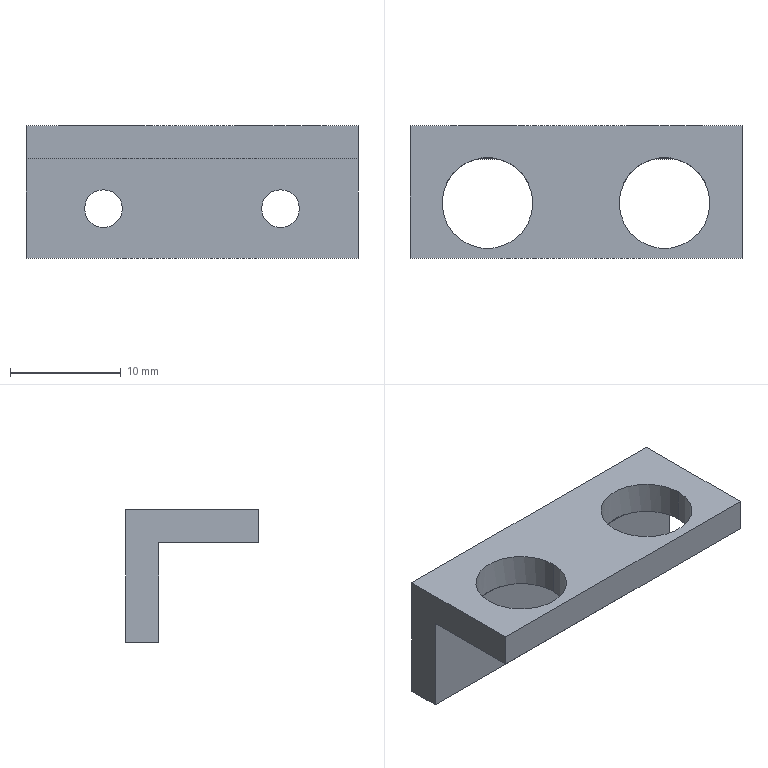NC program | NX | posted with a generic post | part box 30 x 12 x 12 mm
Whole program:
N10 G17 G21 G94 G90
(HOLE_MILLING , TOOL : D4)
N12 T17 M6
N14 G54
N16 G17 G0 G90 X-8. Y-0.998 B0. C0. S5000 M3
N18 G43 Z30. H17
N20 Z0.5
N22 G94 G3 X-7. Y-1.998 R1. F1250.
N24 X-6. Y-0.998 R1.
N26 X-6. Y-0.998 Z0.42 I-2. J0.
N28 X-6. Y-0.998 Z0.34 I-2. J0.
N30 X-6. Y-0.998 Z0.26 I-2. J0.
N32 X-6. Y-0.998 Z0.18 I-2. J0.
N34 X-6. Y-0.998 Z0.1 I-2. J0.
N36 X-6. Y-0.998 Z0.02 I-2. J0.
N38 X-6. Y-0.998 Z-0.06 I-2. J0.
N40 X-6. Y-0.998 Z-0.14 I-2. J0.
N42 X-6. Y-0.998 Z-0.22 I-2. J0.
N44 X-6. Y-0.998 Z-0.3 I-2. J0.
N46 X-6. Y-0.998 Z-0.38 I-2. J0.
N48 X-6. Y-0.998 Z-0.46 I-2. J0.
N50 X-6. Y-0.998 Z-0.54 I-2. J0.
N52 X-6. Y-0.998 Z-0.62 I-2. J0.
N54 X-6. Y-0.998 Z-0.7 I-2. J0.
N56 X-6. Y-0.998 Z-0.78 I-2. J0.
N58 X-6. Y-0.998 Z-0.86 I-2. J0.
N60 X-6. Y-0.998 Z-0.94 I-2. J0.
N62 X-6. Y-0.998 Z-1.02 I-2. J0.
N64 X-6. Y-0.998 Z-1.1 I-2. J0.
N66 X-6. Y-0.998 Z-1.18 I-2. J0.
N68 X-6. Y-0.998 Z-1.26 I-2. J0.
N70 X-6. Y-0.998 Z-1.34 I-2. J0.
N72 X-6. Y-0.998 Z-1.42 I-2. J0.
N74 X-6. Y-0.998 Z-1.5 I-2. J0.
N76 X-6. Y-0.998 Z-1.58 I-2. J0.
N78 X-6. Y-0.998 Z-1.66 I-2. J0.
N80 X-6. Y-0.998 Z-1.74 I-2. J0.
N82 X-6. Y-0.998 Z-1.82 I-2. J0.
N84 X-6. Y-0.998 Z-1.9 I-2. J0.
N86 X-6. Y-0.998 Z-1.98 I-2. J0.
N88 X-6. Y-0.998 Z-2.06 I-2. J0.
N90 X-6. Y-0.998 Z-2.14 I-2. J0.
N92 X-6. Y-0.998 Z-2.22 I-2. J0.
N94 X-6. Y-0.998 Z-2.3 I-2. J0.
N96 X-6. Y-0.998 Z-2.38 I-2. J0.
N98 X-6. Y-0.998 Z-2.46 I-2. J0.
N100 X-6. Y-0.998 Z-2.54 I-2. J0.
N102 X-6. Y-0.998 Z-2.62 I-2. J0.
N104 X-6. Y-0.998 Z-2.7 I-2. J0.
N106 X-6. Y-0.998 Z-2.78 I-2. J0.
N108 X-6. Y-0.998 Z-2.86 I-2. J0.
N110 X-6. Y-0.998 Z-2.94 I-2. J0.
N112 X-8. Y-2.998 Z-3. R-2.
N114 X-6. Y-0.998 R2.
N116 X-8. Y-2.998 R-2.
N118 X-7. Y-1.998 R1.
N120 X-8. Y-0.998 R1.
N122 G0 Z30.
N124 X8.
N126 Z0.5
N128 G3 X9. Y-1.998 R1.
N130 X10. Y-0.998 R1.
N132 X10. Y-0.998 Z0.42 I-2. J0.
N134 X10. Y-0.998 Z0.34 I-2. J0.
N136 X10. Y-0.998 Z0.26 I-2. J0.
N138 X10. Y-0.998 Z0.18 I-2. J0.
N140 X10. Y-0.998 Z0.1 I-2. J0.
N142 X10. Y-0.998 Z0.02 I-2. J0.
N144 X10. Y-0.998 Z-0.06 I-2. J0.
N146 X10. Y-0.998 Z-0.14 I-2. J0.
N148 X10. Y-0.998 Z-0.22 I-2. J0.
N150 X10. Y-0.998 Z-0.3 I-2. J0.
N152 X10. Y-0.998 Z-0.38 I-2. J0.
N154 X10. Y-0.998 Z-0.46 I-2. J0.
N156 X10. Y-0.998 Z-0.54 I-2. J0.
N158 X10. Y-0.998 Z-0.62 I-2. J0.
N160 X10. Y-0.998 Z-0.7 I-2. J0.
N162 X10. Y-0.998 Z-0.78 I-2. J0.
N164 X10. Y-0.998 Z-0.86 I-2. J0.
N166 X10. Y-0.998 Z-0.94 I-2. J0.
N168 X10. Y-0.998 Z-1.02 I-2. J0.
N170 X10. Y-0.998 Z-1.1 I-2. J0.
N172 X10. Y-0.998 Z-1.18 I-2. J0.
N174 X10. Y-0.998 Z-1.26 I-2. J0.
N176 X10. Y-0.998 Z-1.34 I-2. J0.
N178 X10. Y-0.998 Z-1.42 I-2. J0.
N180 X10. Y-0.998 Z-1.5 I-2. J0.
N182 X10. Y-0.998 Z-1.58 I-2. J0.
N184 X10. Y-0.998 Z-1.66 I-2. J0.
N186 X10. Y-0.998 Z-1.74 I-2. J0.
N188 X10. Y-0.998 Z-1.82 I-2. J0.
N190 X10. Y-0.998 Z-1.9 I-2. J0.
N192 X10. Y-0.998 Z-1.98 I-2. J0.
N194 X10. Y-0.998 Z-2.06 I-2. J0.
N196 X10. Y-0.998 Z-2.14 I-2. J0.
N198 X10. Y-0.998 Z-2.22 I-2. J0.
N200 X10. Y-0.998 Z-2.3 I-2. J0.
N202 X10. Y-0.998 Z-2.38 I-2. J0.
N204 X10. Y-0.998 Z-2.46 I-2. J0.
N206 X10. Y-0.998 Z-2.54 I-2. J0.
N208 X10. Y-0.998 Z-2.62 I-2. J0.
N210 X10. Y-0.998 Z-2.7 I-2. J0.
N212 X10. Y-0.998 Z-2.78 I-2. J0.
N214 X10. Y-0.998 Z-2.86 I-2. J0.
N216 X10. Y-0.998 Z-2.94 I-2. J0.
N218 X8. Y-2.998 Z-3. R-2.
N220 X10. Y-0.998 R2.
N222 X8. Y-2.998 R-2.
N224 X9. Y-1.998 R1.
N226 X8. Y-0.998 R1.
N228 G0 Z30.
N230 M5
N232 M2